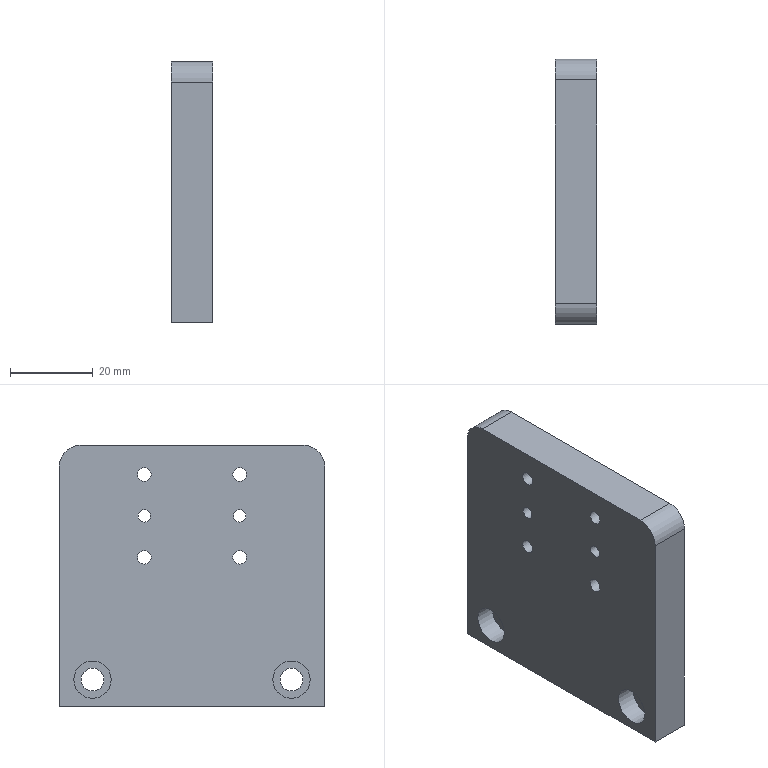Part | STEP file | ROTATION MC_NEW VER-0610_552 | 1 solid | 183 faces | box 10 x 64 x 63 mm | volume 38849 mm3 | plane 114 | spline 57 | cylinder 12 | commonest cylinder face diameters 3.3 x4 3 x2 5.5 x2 9 x2 10 x2